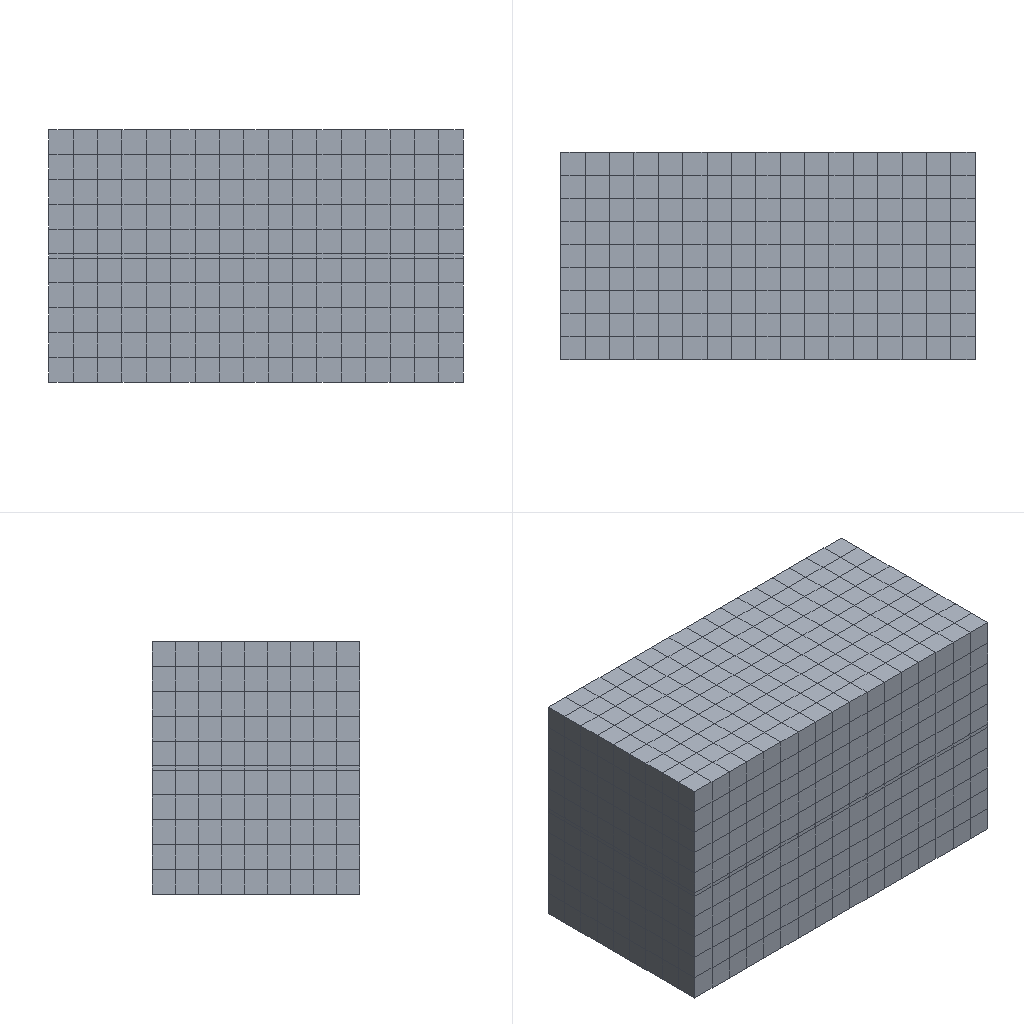Simulation study | ansys workbench
Set-up summary:
category,name,step,type,value,unit,region
solver,ansys_workbench
units,mm-N-s-tonne (MPa),,stated,"/units,MPA"
analysis,deck-1/LS1,,transient thermal
load_step,deck-1/LS1,deck-1/LS1,transient thermal,nsubst=100; time=1
load_step,deck-1/LS2,deck-1/LS2,transient thermal,nsubst=100; time=2
load_step,deck-1/LS3,deck-1/LS3,transient thermal,nsubst=100; time=3
load_step,deck-1/LS4,deck-1/LS4,transient thermal,nsubst=100; time=4
load_step,deck-1/LS5,deck-1/LS5,transient thermal,nsubst=100; time=5
analysis,deck-2/LS1,,transient
load_step,deck-2/LS1,deck-2/LS1,transient,time=1
mesh,deck-1.dat,,nodes,9148
mesh,deck-1.dat,,elements,5240
element_type,SURF152,,,2333,,deck-1.dat
element_type,SOLID279,,,1683,,deck-1.dat
element_type,TARGE170,,,612,,deck-1.dat
element_type,CONTA174,,,612,,deck-1.dat
mesh,deck-2.dat,,nodes,9148
mesh,deck-2.dat,,elements,2907
element_type,SOLID186,,,1683,,deck-2.dat
element_type,TARGE170,,,612,,deck-2.dat
element_type,CONTA174,,,612,,deck-2.dat
material,SI3N4,,E,300000,tonne s^-2 mm^-1
material,SI3N4,,nu,0.27
material,SI3N4,,density,3.2e-09,tonne mm^-3
material,SI3N4,,conductivity,20,tonne mm s^-3 C^-1
material,SI3N4,,specific_heat,7.5e+08,mm^2 s^-2 C^-1
material,SI3N4,,cte,3.5e-06,C^-1
material,Titanium Alloy,,E,110000,tonne s^-2 mm^-1
material,Titanium Alloy,,nu,0.34
material,Titanium Alloy,,density,4.51e-09,tonne mm^-3
material,Titanium Alloy,,conductivity,19,tonne mm s^-3 C^-1
material,Titanium Alloy,,specific_heat,5.3e+08,mm^2 s^-2 C^-1
material,Titanium Alloy,,permeability,1
material,Titanium Alloy,,resistivity,0.0017,ohm mm
material,AG-CU-TI,,E,75000,tonne s^-2 mm^-1
material,AG-CU-TI,,nu,0.35
material,AG-CU-TI,,density,9.8e-09,tonne mm^-3
material,AG-CU-TI,,conductivity,110,tonne mm s^-3 C^-1
material,AG-CU-TI,,specific_heat,4.2e+08,mm^2 s^-2 C^-1
load,Define Uniform Initial temperature,deck-1/model,body load temp,25,,all
load,"Create ""?""",deck-1/LS1,heat flux,200000,,SURF152 #8
load,"Create ""______""",deck-1/LS1,convection,0.0124,,SURF152 #9
load,"Create Imported Load ""________""",deck-2/LS1,body load temp,,,all
bc,,deck-1/LS1,temperature,25 [dofs=TEMP],,node list
bc,Frictionless Supports Y,deck-2/model,fixed,[dofs=UY],,_FRICSUY
bc,Constant Zero Displacement X,deck-2/model,fixed,[dofs=UX],,_DISPZEROUX
bc,Constant Zero Displacement Y,deck-2/model,fixed,[dofs=UY],,_DISPZEROUY
bc,Constant Zero Displacement Z,deck-2/model,fixed,[dofs=UZ],,_DISPZEROUZ
contact,Contact Region,,bonded (always),element=CONTA174
contact,Contact Region 2,,bonded (always),element=CONTA174
contact,Contact Region,,bonded (always),element=CONTA174
contact,Contact Region 2,,bonded (always),element=CONTA174
named_set,_FRICSUY,,node,688
named_set,_DISPZEROUX,,node,76
named_set,_DISPZEROUY,,node,72
named_set,_DISPZEROUZ,,node,76
named_set,_LV_54__SELECTION,,node,9148
Results summary:
result,analyses[0].index,,,1
result,analyses[0].system,,,SYS
result,analyses[0].deck,,,deck-1.dat
result,analyses[0].solve_status,,,completed
result,analyses[0].analysis_type,,,static
result,analyses[0].physics,,,thermal
result,analyses[0].unit_system,,,"NMM: mm, ton, N, s, mV, mA, degC"
result,analyses[0].n_sets,,,68
result,analyses[0].load_steps[0].set,set=16,,16
result,analyses[0].load_steps[0].time_or_freq,set=16,,1
result,analyses[0].load_steps[0].max_temperature,set=16,,1151.67
result,analyses[0].load_steps[0].min_temperature,set=16,,25
result,analyses[0].load_steps[1].set,set=29,,29
result,analyses[0].load_steps[1].time_or_freq,set=29,,2
result,analyses[0].load_steps[1].max_temperature,set=29,,1416.85
result,analyses[0].load_steps[1].min_temperature,set=29,,25
result,analyses[0].load_steps[2].set,set=42,,42
result,analyses[0].load_steps[2].time_or_freq,set=42,,3
result,analyses[0].load_steps[2].max_temperature,set=42,,1662.37
result,analyses[0].load_steps[2].min_temperature,set=42,,25
result,analyses[0].load_steps[3].set,set=55,,55
result,analyses[0].load_steps[3].time_or_freq,set=55,,4
result,analyses[0].load_steps[3].max_temperature,set=55,,1886.33
result,analyses[0].load_steps[3].min_temperature,set=55,,25
result,analyses[0].load_steps[4].set,set=68,,68
result,analyses[0].load_steps[4].time_or_freq,set=68,,5
result,analyses[0].load_steps[4].max_temperature,set=68,,2081.15
result,analyses[0].load_steps[4].min_temperature,set=68,,25
result,analyses[1].index,,,2
result,analyses[1].system,,,SYS-1
result,analyses[1].deck,,,deck-2.dat
result,analyses[1].solve_status,,,completed
result,analyses[1].analysis_type,,,static
result,analyses[1].physics,,,mechanical
result,analyses[1].unit_system,,,"NMM: mm, ton, N, s, mV, mA, degC"
result,analyses[1].n_sets,,,199
result,analyses[1].load_steps[0].set,set=199,,199
result,analyses[1].load_steps[0].time_or_freq,set=199,,1
result,analyses[1].load_steps[0].max_displacement_magnitude,set=199,,0.02207
result,analyses[1].load_steps[0].max_von_mises_nodal,set=199,,6991.78
result,analyses[1].load_steps[0].reaction_force_sum_xyz[1],set=199,,-5.25802e-12
result,analyses[1].load_steps[0].reaction_force_sum_xyz[2],set=199,,0.0001633
result,analyses[1].load_steps[0].reaction_force_sum_xyz[3],set=199,,8.81001e-05
result,geometry_export[0][0],,,.step
result,geometry_export[0][1],,,ok
result,geometry_export[0][2],,,3